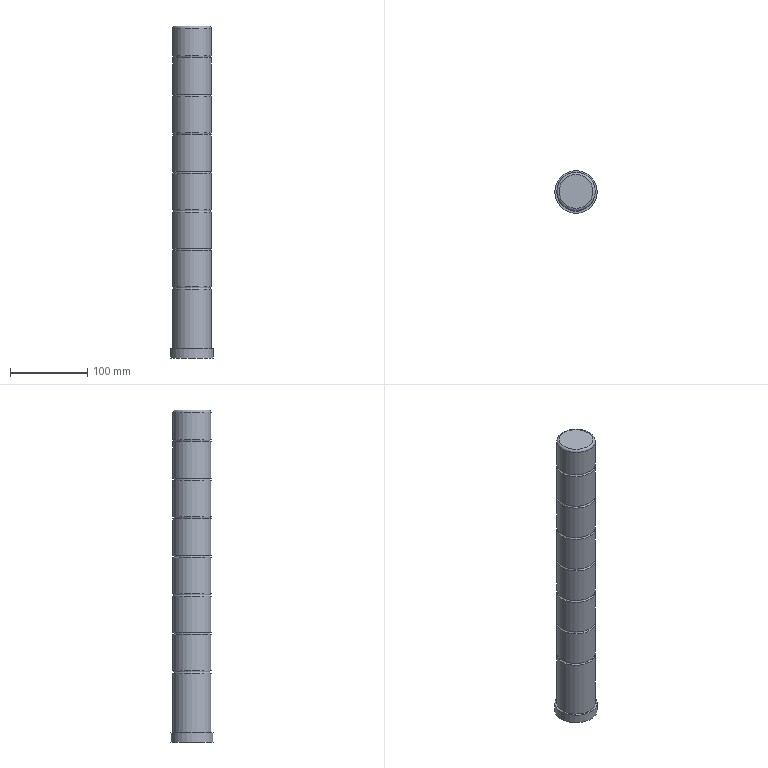Part | STEP file | solid 125 | 1 solid | 20 faces | box 55 x 55 x 431 mm | volume 847132 mm3 | cylinder 9 | torus 8 | plane 3 | commonest cylinder face diameters 50 x8 55 x1